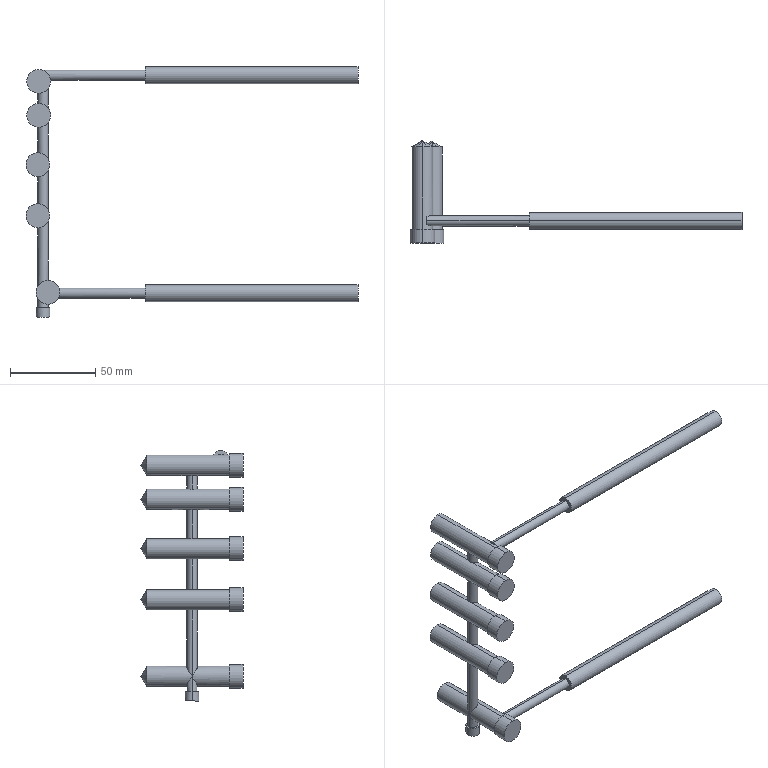Part | STEP file | 1 solid | 70 faces | box 195 x 60 x 147.144 mm | volume 59737 mm3 | cylinder 43 | plane 17 | cone 10 | commonest cylinder face diameters 6 x14 12 x13 14 x10 10 x4 8 x2